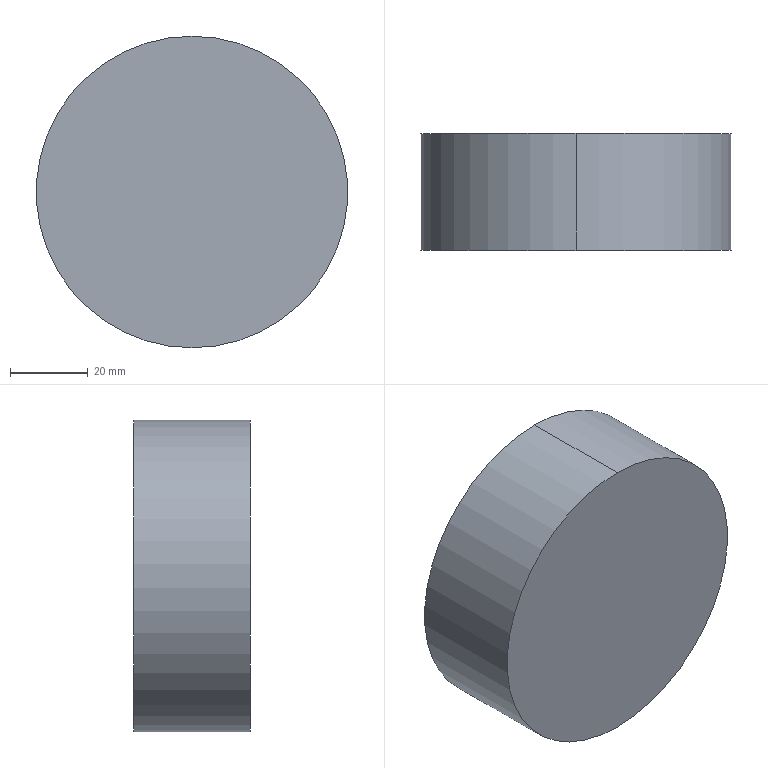Part | 1 solid | 4 faces | box 80 x 30 x 80 mm | volume 150796 mm3 | cylinder 2 | plane 2 | commonest cylinder face diameters 80 x2
STEP:
#1=CARTESIAN_POINT('',(0.,0.,0.));
#2=DIRECTION('',(0.,0.,1.));
#3=DIRECTION('',(1.,0.,0.));
#4=AXIS2_PLACEMENT_3D('',#1,#2,#3);
#5=CARTESIAN_POINT('',(-239.028,-196.5,-340.55));
#6=VERTEX_POINT('',#5);
#7=CARTESIAN_POINT('',(-239.028,-166.5,-340.55));
#8=VERTEX_POINT('',#7);
#9=CARTESIAN_POINT('',(-239.028,-196.5,-340.55));
#10=DIRECTION('',(0.,1.,0.));
#11=VECTOR('',#10,1.);
#12=LINE('',#9,#11);
#13=CARTESIAN_POINT('',(-239.028,-196.5,-300.55));
#14=DIRECTION('',(0.,1.,0.));
#15=DIRECTION('',(1.,0.,0.));
#16=AXIS2_PLACEMENT_3D('',#13,#14,#15);
#17=CYLINDRICAL_SURFACE('',#16,40.);
#18=CARTESIAN_POINT('',(1.571,0.));
#19=DIRECTION('',(0.,1.));
#20=VECTOR('',#19,1.);
#21=LINE('',#18,#20);
#22=(GEOMETRIC_REPRESENTATION_CONTEXT(2)PARAMETRIC_REPRESENTATION_CONTEXT()REPRESENTATION_CONTEXT('',''));
#23=DEFINITIONAL_REPRESENTATION('',(#21),#22);
#24=PCURVE('',#17,#23);
#25=CARTESIAN_POINT('',(-239.028,-196.5,-300.55));
#26=DIRECTION('',(0.,1.,0.));
#27=DIRECTION('',(-1.,0.,0.));
#28=AXIS2_PLACEMENT_3D('',#25,#26,#27);
#29=CYLINDRICAL_SURFACE('',#28,40.);
#30=CARTESIAN_POINT('',(4.712,0.));
#31=DIRECTION('',(0.,1.));
#32=VECTOR('',#31,1.);
#33=LINE('',#30,#32);
#34=(GEOMETRIC_REPRESENTATION_CONTEXT(2)PARAMETRIC_REPRESENTATION_CONTEXT()REPRESENTATION_CONTEXT('',''));
#35=DEFINITIONAL_REPRESENTATION('',(#33),#34);
#36=PCURVE('',#29,#35);
#37=SURFACE_CURVE('',#12,(#24,#36),.PCURVE_S1.);
#38=EDGE_CURVE('',#6,#8,#37,.T.);
#39=ORIENTED_EDGE('',*,*,#38,.F.);
#40=CARTESIAN_POINT('',(-239.028,-196.5,-260.55));
#41=VERTEX_POINT('',#40);
#42=CARTESIAN_POINT('',(-239.028,-196.5,-300.55));
#43=DIRECTION('',(0.,1.,0.));
#44=DIRECTION('',(0.,0.,1.));
#45=AXIS2_PLACEMENT_3D('',#42,#43,#44);
#46=CIRCLE('',#45,40.);
#47=CARTESIAN_POINT('',(-1.571,0.));
#48=DIRECTION('',(1.,0.));
#49=VECTOR('',#48,1.);
#50=LINE('',#47,#49);
#51=(GEOMETRIC_REPRESENTATION_CONTEXT(2)PARAMETRIC_REPRESENTATION_CONTEXT()REPRESENTATION_CONTEXT('',''));
#52=DEFINITIONAL_REPRESENTATION('',(#50),#51);
#53=PCURVE('',#17,#52);
#54=CARTESIAN_POINT('',(-239.028,-196.5,-300.55));
#55=DIRECTION('',(0.,1.,0.));
#56=DIRECTION('',(0.,0.,1.));
#57=AXIS2_PLACEMENT_3D('',#54,#55,#56);
#58=PLANE('',#57);
#59=CARTESIAN_POINT('',(0.,0.));
#60=DIRECTION('',(1.,0.));
#61=AXIS2_PLACEMENT_2D('',#59,#60);
#62=CIRCLE('',#61,40.);
#63=(GEOMETRIC_REPRESENTATION_CONTEXT(2)PARAMETRIC_REPRESENTATION_CONTEXT()REPRESENTATION_CONTEXT('',''));
#64=DEFINITIONAL_REPRESENTATION('',(#62),#63);
#65=PCURVE('',#58,#64);
#66=SURFACE_CURVE('',#46,(#53,#65),.PCURVE_S1.);
#67=EDGE_CURVE('',#6,#41,#66,.T.);
#68=ORIENTED_EDGE('',*,*,#67,.T.);
#69=CARTESIAN_POINT('',(-239.028,-166.5,-260.55));
#70=VERTEX_POINT('',#69);
#71=CARTESIAN_POINT('',(-239.028,-196.5,-260.55));
#72=DIRECTION('',(0.,1.,0.));
#73=VECTOR('',#72,1.);
#74=LINE('',#71,#73);
#75=CARTESIAN_POINT('',(4.712,0.));
#76=DIRECTION('',(0.,1.));
#77=VECTOR('',#76,1.);
#78=LINE('',#75,#77);
#79=(GEOMETRIC_REPRESENTATION_CONTEXT(2)PARAMETRIC_REPRESENTATION_CONTEXT()REPRESENTATION_CONTEXT('',''));
#80=DEFINITIONAL_REPRESENTATION('',(#78),#79);
#81=PCURVE('',#17,#80);
#82=CARTESIAN_POINT('',(1.571,0.));
#83=DIRECTION('',(0.,1.));
#84=VECTOR('',#83,1.);
#85=LINE('',#82,#84);
#86=(GEOMETRIC_REPRESENTATION_CONTEXT(2)PARAMETRIC_REPRESENTATION_CONTEXT()REPRESENTATION_CONTEXT('',''));
#87=DEFINITIONAL_REPRESENTATION('',(#85),#86);
#88=PCURVE('',#29,#87);
#89=SURFACE_CURVE('',#74,(#81,#88),.PCURVE_S1.);
#90=EDGE_CURVE('',#41,#70,#89,.T.);
#91=ORIENTED_EDGE('',*,*,#90,.T.);
#92=CARTESIAN_POINT('',(-239.028,-166.5,-300.55));
#93=DIRECTION('',(0.,1.,0.));
#94=DIRECTION('',(0.,0.,1.));
#95=AXIS2_PLACEMENT_3D('',#92,#93,#94);
#96=CIRCLE('',#95,40.);
#97=CARTESIAN_POINT('',(-1.571,30.));
#98=DIRECTION('',(1.,0.));
#99=VECTOR('',#98,1.);
#100=LINE('',#97,#99);
#101=(GEOMETRIC_REPRESENTATION_CONTEXT(2)PARAMETRIC_REPRESENTATION_CONTEXT()REPRESENTATION_CONTEXT('',''));
#102=DEFINITIONAL_REPRESENTATION('',(#100),#101);
#103=PCURVE('',#17,#102);
#104=CARTESIAN_POINT('',(-239.028,-166.5,-300.55));
#105=DIRECTION('',(0.,1.,0.));
#106=DIRECTION('',(0.,0.,1.));
#107=AXIS2_PLACEMENT_3D('',#104,#105,#106);
#108=PLANE('',#107);
#109=CARTESIAN_POINT('',(0.,0.));
#110=DIRECTION('',(1.,0.));
#111=AXIS2_PLACEMENT_2D('',#109,#110);
#112=CIRCLE('',#111,40.);
#113=(GEOMETRIC_REPRESENTATION_CONTEXT(2)PARAMETRIC_REPRESENTATION_CONTEXT()REPRESENTATION_CONTEXT('',''));
#114=DEFINITIONAL_REPRESENTATION('',(#112),#113);
#115=PCURVE('',#108,#114);
#116=SURFACE_CURVE('',#96,(#103,#115),.PCURVE_S1.);
#117=EDGE_CURVE('',#8,#70,#116,.T.);
#118=ORIENTED_EDGE('',*,*,#117,.F.);
#119=EDGE_LOOP('',(#39,#68,#91,#118));
#120=FACE_BOUND('',#119,.T.);
#121=ADVANCED_FACE('',(#120),#17,.T.);
#122=CARTESIAN_POINT('',(-239.028,-166.5,-300.55));
#123=DIRECTION('',(0.,1.,0.));
#124=DIRECTION('',(0.,0.,1.));
#125=AXIS2_PLACEMENT_3D('',#122,#123,#124);
#126=CIRCLE('',#125,40.);
#127=CARTESIAN_POINT('',(0.,0.));
#128=DIRECTION('',(1.,0.));
#129=AXIS2_PLACEMENT_2D('',#127,#128);
#130=CIRCLE('',#129,40.);
#131=(GEOMETRIC_REPRESENTATION_CONTEXT(2)PARAMETRIC_REPRESENTATION_CONTEXT()REPRESENTATION_CONTEXT('',''));
#132=DEFINITIONAL_REPRESENTATION('',(#130),#131);
#133=PCURVE('',#108,#132);
#134=CARTESIAN_POINT('',(1.571,30.));
#135=DIRECTION('',(1.,0.));
#136=VECTOR('',#135,1.);
#137=LINE('',#134,#136);
#138=(GEOMETRIC_REPRESENTATION_CONTEXT(2)PARAMETRIC_REPRESENTATION_CONTEXT()REPRESENTATION_CONTEXT('',''));
#139=DEFINITIONAL_REPRESENTATION('',(#137),#138);
#140=PCURVE('',#29,#139);
#141=SURFACE_CURVE('',#126,(#133,#140),.PCURVE_S1.);
#142=EDGE_CURVE('',#70,#8,#141,.T.);
#143=ORIENTED_EDGE('',*,*,#142,.T.);
#144=ORIENTED_EDGE('',*,*,#117,.T.);
#145=EDGE_LOOP('',(#143,#144));
#146=FACE_BOUND('',#145,.T.);
#147=ADVANCED_FACE('',(#146),#108,.T.);
#148=ORIENTED_EDGE('',*,*,#67,.F.);
#149=CARTESIAN_POINT('',(-239.028,-196.5,-300.55));
#150=DIRECTION('',(0.,1.,0.));
#151=DIRECTION('',(0.,0.,1.));
#152=AXIS2_PLACEMENT_3D('',#149,#150,#151);
#153=CIRCLE('',#152,40.);
#154=CARTESIAN_POINT('',(0.,0.));
#155=DIRECTION('',(1.,0.));
#156=AXIS2_PLACEMENT_2D('',#154,#155);
#157=CIRCLE('',#156,40.);
#158=(GEOMETRIC_REPRESENTATION_CONTEXT(2)PARAMETRIC_REPRESENTATION_CONTEXT()REPRESENTATION_CONTEXT('',''));
#159=DEFINITIONAL_REPRESENTATION('',(#157),#158);
#160=PCURVE('',#58,#159);
#161=CARTESIAN_POINT('',(1.571,0.));
#162=DIRECTION('',(1.,0.));
#163=VECTOR('',#162,1.);
#164=LINE('',#161,#163);
#165=(GEOMETRIC_REPRESENTATION_CONTEXT(2)PARAMETRIC_REPRESENTATION_CONTEXT()REPRESENTATION_CONTEXT('',''));
#166=DEFINITIONAL_REPRESENTATION('',(#164),#165);
#167=PCURVE('',#29,#166);
#168=SURFACE_CURVE('',#153,(#160,#167),.PCURVE_S1.);
#169=EDGE_CURVE('',#41,#6,#168,.T.);
#170=ORIENTED_EDGE('',*,*,#169,.F.);
#171=EDGE_LOOP('',(#148,#170));
#172=FACE_BOUND('',#171,.T.);
#173=ADVANCED_FACE('',(#172),#58,.F.);
#174=ORIENTED_EDGE('',*,*,#38,.T.);
#175=ORIENTED_EDGE('',*,*,#142,.F.);
#176=ORIENTED_EDGE('',*,*,#90,.F.);
#177=ORIENTED_EDGE('',*,*,#169,.T.);
#178=EDGE_LOOP('',(#174,#175,#176,#177));
#179=FACE_BOUND('',#178,.T.);
#180=ADVANCED_FACE('',(#179),#29,.T.);
#181=CLOSED_SHELL('',(#121,#147,#173,#180));
#182=MANIFOLD_SOLID_BREP('',#181);
#183=(LENGTH_UNIT()NAMED_UNIT(*)SI_UNIT(.MILLI.,.METRE.));
#184=UNCERTAINTY_MEASURE_WITH_UNIT(LENGTH_MEASURE(0.0000001),#183,'','');
#185=(NAMED_UNIT(*)PLANE_ANGLE_UNIT()SI_UNIT($,.RADIAN.));
#186=(NAMED_UNIT(*)SI_UNIT($,.STERADIAN.)SOLID_ANGLE_UNIT());
#187=(GEOMETRIC_REPRESENTATION_CONTEXT(3)GLOBAL_UNCERTAINTY_ASSIGNED_CONTEXT((#184))GLOBAL_UNIT_ASSIGNED_CONTEXT((#183,#185,#186))REPRESENTATION_CONTEXT('',''));
#188=ADVANCED_BREP_SHAPE_REPRESENTATION('',(#4,#182),#187);